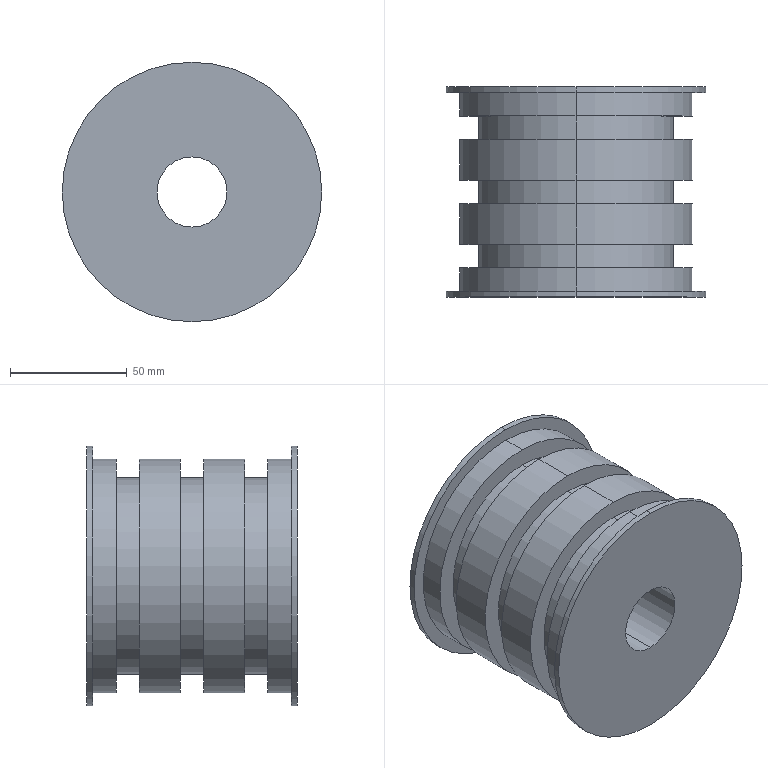Part | STEP file | 012-6-07-016 | 1 solid | 30 faces | box 111 x 90 x 111 mm | volume 582989 mm3 | cylinder 20 | plane 10 | commonest cylinder face diameters 100 x8 84 x6 111 x4 30 x2